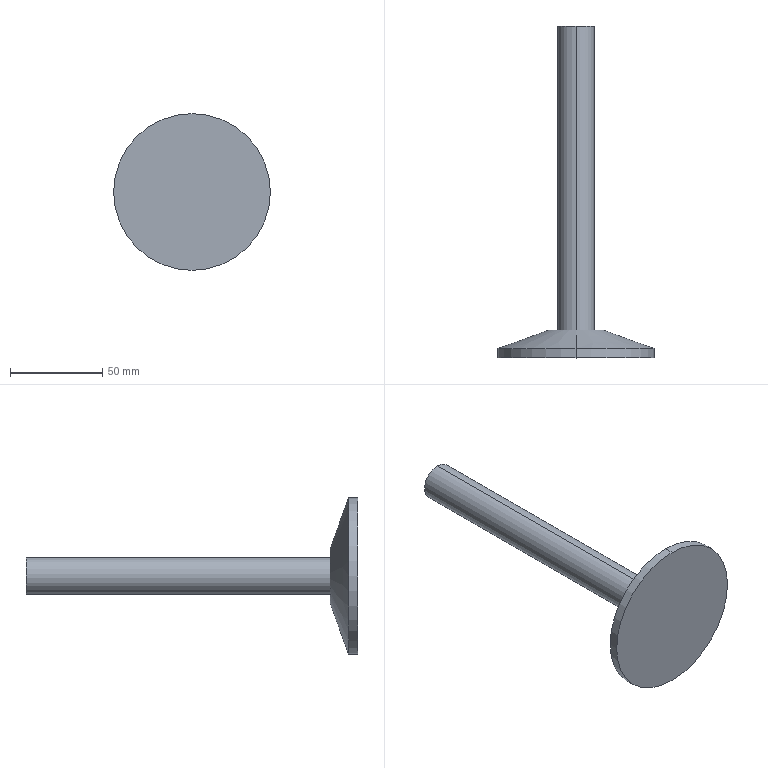Part | SolidWorks | features BaseBody 1 | 1 solid | 9 faces | box 85 x 180 x 85 mm | volume 108156 mm3 | cylinder 4 | plane 3 | cone 2 | commonest cylinder face diameters 20 x2 85 x2
STEP:
#1=CARTESIAN_POINT('',(0.,0.,42.5));
#2=VERTEX_POINT('',#1);
#3=CARTESIAN_POINT('',(0.,0.,-42.5));
#4=VERTEX_POINT('',#3);
#5=CARTESIAN_POINT('',(0.,0.,0.));
#6=DIRECTION('',(0.,1.,0.));
#7=DIRECTION('',(0.,0.,1.));
#8=AXIS2_PLACEMENT_3D('',#5,#6,#7);
#9=CIRCLE('',#8,42.5);
#10=EDGE_CURVE('',#2,#4,#9,.T.);
#11=ORIENTED_EDGE('',*,*,#10,.T.);
#12=CARTESIAN_POINT('',(0.,5.,-42.5));
#13=VERTEX_POINT('',#12);
#14=CARTESIAN_POINT('',(0.,86.546,-42.5));
#15=DIRECTION('',(0.,1.,0.));
#16=VECTOR('',#15,1000.);
#17=LINE('',#14,#16);
#18=EDGE_CURVE('',#4,#13,#17,.T.);
#19=ORIENTED_EDGE('',*,*,#18,.T.);
#20=CARTESIAN_POINT('',(0.,5.,42.5));
#21=VERTEX_POINT('',#20);
#22=CARTESIAN_POINT('',(0.,5.,0.));
#23=DIRECTION('',(0.,-1.,0.));
#24=DIRECTION('',(0.,0.,1.));
#25=AXIS2_PLACEMENT_3D('',#22,#23,#24);
#26=CIRCLE('',#25,42.5);
#27=EDGE_CURVE('',#13,#21,#26,.T.);
#28=ORIENTED_EDGE('',*,*,#27,.T.);
#29=CARTESIAN_POINT('',(0.,86.546,42.5));
#30=DIRECTION('',(0.,1.,0.));
#31=VECTOR('',#30,1000.);
#32=LINE('',#29,#31);
#33=EDGE_CURVE('',#2,#21,#32,.T.);
#34=ORIENTED_EDGE('',*,*,#33,.F.);
#35=EDGE_LOOP('',(#11,#19,#28,#34));
#36=FACE_OUTER_BOUND('',#35,.T.);
#37=CARTESIAN_POINT('',(0.,86.546,0.));
#38=DIRECTION('',(0.,1.,0.));
#39=DIRECTION('',(0.,0.,1.));
#40=AXIS2_PLACEMENT_3D('',#37,#38,#39);
#41=CYLINDRICAL_SURFACE('',#40,42.5);
#42=ADVANCED_FACE('',(#36),#41,.T.);
#43=CARTESIAN_POINT('',(0.,15.,-15.));
#44=VERTEX_POINT('',#43);
#45=CARTESIAN_POINT('',(0.,15.,15.));
#46=VERTEX_POINT('',#45);
#47=CARTESIAN_POINT('',(0.,15.,0.));
#48=DIRECTION('',(0.,-1.,0.));
#49=DIRECTION('',(0.,0.,-1.));
#50=AXIS2_PLACEMENT_3D('',#47,#48,#49);
#51=CIRCLE('',#50,15.);
#52=EDGE_CURVE('',#44,#46,#51,.T.);
#53=ORIENTED_EDGE('',*,*,#52,.T.);
#54=CARTESIAN_POINT('',(0.,5.,42.5));
#55=DIRECTION('',(0.,-0.3417,0.9398));
#56=VECTOR('',#55,1000.);
#57=LINE('',#54,#56);
#58=EDGE_CURVE('',#46,#21,#57,.T.);
#59=ORIENTED_EDGE('',*,*,#58,.T.);
#60=ORIENTED_EDGE('',*,*,#27,.F.);
#61=CARTESIAN_POINT('',(0.,5.,-42.5));
#62=DIRECTION('',(0.,-0.3417,-0.9398));
#63=VECTOR('',#62,1000.);
#64=LINE('',#61,#63);
#65=EDGE_CURVE('',#44,#13,#64,.T.);
#66=ORIENTED_EDGE('',*,*,#65,.F.);
#67=EDGE_LOOP('',(#53,#59,#60,#66));
#68=FACE_OUTER_BOUND('',#67,.T.);
#69=CARTESIAN_POINT('',(0.,5.,0.));
#70=DIRECTION('',(0.,-1.,0.));
#71=DIRECTION('',(0.,0.,-1.));
#72=AXIS2_PLACEMENT_3D('',#69,#70,#71);
#73=CONICAL_SURFACE('',#72,42.5,1.222);
#74=ADVANCED_FACE('',(#68),#73,.T.);
#75=CARTESIAN_POINT('',(0.,15.,10.));
#76=VERTEX_POINT('',#75);
#77=CARTESIAN_POINT('',(0.,15.,-10.));
#78=VERTEX_POINT('',#77);
#79=CARTESIAN_POINT('',(0.,15.,0.));
#80=DIRECTION('',(0.,1.,0.));
#81=DIRECTION('',(0.,0.,1.));
#82=AXIS2_PLACEMENT_3D('',#79,#80,#81);
#83=CIRCLE('',#82,10.);
#84=EDGE_CURVE('',#76,#78,#83,.T.);
#85=ORIENTED_EDGE('',*,*,#84,.T.);
#86=CARTESIAN_POINT('',(0.,180.,-10.));
#87=VERTEX_POINT('',#86);
#88=CARTESIAN_POINT('',(0.,86.546,-10.));
#89=DIRECTION('',(0.,1.,0.));
#90=VECTOR('',#89,1000.);
#91=LINE('',#88,#90);
#92=EDGE_CURVE('',#78,#87,#91,.T.);
#93=ORIENTED_EDGE('',*,*,#92,.T.);
#94=CARTESIAN_POINT('',(0.,180.,10.));
#95=VERTEX_POINT('',#94);
#96=CARTESIAN_POINT('',(0.,180.,0.));
#97=DIRECTION('',(0.,-1.,0.));
#98=DIRECTION('',(0.,0.,1.));
#99=AXIS2_PLACEMENT_3D('',#96,#97,#98);
#100=CIRCLE('',#99,10.);
#101=EDGE_CURVE('',#87,#95,#100,.T.);
#102=ORIENTED_EDGE('',*,*,#101,.T.);
#103=CARTESIAN_POINT('',(0.,86.546,10.));
#104=DIRECTION('',(0.,1.,0.));
#105=VECTOR('',#104,1000.);
#106=LINE('',#103,#105);
#107=EDGE_CURVE('',#76,#95,#106,.T.);
#108=ORIENTED_EDGE('',*,*,#107,.F.);
#109=EDGE_LOOP('',(#85,#93,#102,#108));
#110=FACE_OUTER_BOUND('',#109,.T.);
#111=CARTESIAN_POINT('',(0.,86.546,0.));
#112=DIRECTION('',(0.,1.,0.));
#113=DIRECTION('',(0.,0.,1.));
#114=AXIS2_PLACEMENT_3D('',#111,#112,#113);
#115=CYLINDRICAL_SURFACE('',#114,10.);
#116=ADVANCED_FACE('',(#110),#115,.T.);
#117=ORIENTED_EDGE('',*,*,#10,.F.);
#118=CARTESIAN_POINT('',(0.,0.,0.));
#119=DIRECTION('',(0.,1.,0.));
#120=DIRECTION('',(0.,0.,1.));
#121=AXIS2_PLACEMENT_3D('',#118,#119,#120);
#122=CIRCLE('',#121,42.5);
#123=EDGE_CURVE('',#4,#2,#122,.T.);
#124=ORIENTED_EDGE('',*,*,#123,.F.);
#125=EDGE_LOOP('',(#117,#124));
#126=FACE_OUTER_BOUND('',#125,.T.);
#127=CARTESIAN_POINT('',(0.,0.,0.));
#128=DIRECTION('',(0.,1.,0.));
#129=DIRECTION('',(0.,0.,1.));
#130=AXIS2_PLACEMENT_3D('',#127,#128,#129);
#131=PLANE('',#130);
#132=ADVANCED_FACE('',(#126),#131,.F.);
#133=ORIENTED_EDGE('',*,*,#18,.F.);
#134=ORIENTED_EDGE('',*,*,#123,.T.);
#135=ORIENTED_EDGE('',*,*,#33,.T.);
#136=CARTESIAN_POINT('',(0.,5.,0.));
#137=DIRECTION('',(0.,-1.,0.));
#138=DIRECTION('',(0.,0.,1.));
#139=AXIS2_PLACEMENT_3D('',#136,#137,#138);
#140=CIRCLE('',#139,42.5);
#141=EDGE_CURVE('',#21,#13,#140,.T.);
#142=ORIENTED_EDGE('',*,*,#141,.T.);
#143=EDGE_LOOP('',(#133,#134,#135,#142));
#144=FACE_OUTER_BOUND('',#143,.T.);
#145=CARTESIAN_POINT('',(0.,86.546,0.));
#146=DIRECTION('',(0.,1.,0.));
#147=DIRECTION('',(0.,0.,1.));
#148=AXIS2_PLACEMENT_3D('',#145,#146,#147);
#149=CYLINDRICAL_SURFACE('',#148,42.5);
#150=ADVANCED_FACE('',(#144),#149,.T.);
#151=ORIENTED_EDGE('',*,*,#58,.F.);
#152=CARTESIAN_POINT('',(0.,15.,0.));
#153=DIRECTION('',(0.,-1.,0.));
#154=DIRECTION('',(0.,0.,-1.));
#155=AXIS2_PLACEMENT_3D('',#152,#153,#154);
#156=CIRCLE('',#155,15.);
#157=EDGE_CURVE('',#46,#44,#156,.T.);
#158=ORIENTED_EDGE('',*,*,#157,.T.);
#159=ORIENTED_EDGE('',*,*,#65,.T.);
#160=ORIENTED_EDGE('',*,*,#141,.F.);
#161=EDGE_LOOP('',(#151,#158,#159,#160));
#162=FACE_OUTER_BOUND('',#161,.T.);
#163=CARTESIAN_POINT('',(0.,5.,0.));
#164=DIRECTION('',(0.,-1.,0.));
#165=DIRECTION('',(0.,0.,-1.));
#166=AXIS2_PLACEMENT_3D('',#163,#164,#165);
#167=CONICAL_SURFACE('',#166,42.5,1.222);
#168=ADVANCED_FACE('',(#162),#167,.T.);
#169=ORIENTED_EDGE('',*,*,#52,.F.);
#170=ORIENTED_EDGE('',*,*,#157,.F.);
#171=EDGE_LOOP('',(#169,#170));
#172=FACE_OUTER_BOUND('',#171,.T.);
#173=ORIENTED_EDGE('',*,*,#84,.F.);
#174=CARTESIAN_POINT('',(0.,15.,0.));
#175=DIRECTION('',(0.,1.,0.));
#176=DIRECTION('',(0.,0.,1.));
#177=AXIS2_PLACEMENT_3D('',#174,#175,#176);
#178=CIRCLE('',#177,10.);
#179=EDGE_CURVE('',#78,#76,#178,.T.);
#180=ORIENTED_EDGE('',*,*,#179,.F.);
#181=EDGE_LOOP('',(#173,#180));
#182=FACE_BOUND('',#181,.T.);
#183=CARTESIAN_POINT('',(15.,15.,0.));
#184=DIRECTION('',(0.,-1.,0.));
#185=DIRECTION('',(0.,0.,-1.));
#186=AXIS2_PLACEMENT_3D('',#183,#184,#185);
#187=PLANE('',#186);
#188=ADVANCED_FACE('',(#172,#182),#187,.F.);
#189=ORIENTED_EDGE('',*,*,#92,.F.);
#190=ORIENTED_EDGE('',*,*,#179,.T.);
#191=ORIENTED_EDGE('',*,*,#107,.T.);
#192=CARTESIAN_POINT('',(0.,180.,0.));
#193=DIRECTION('',(0.,-1.,0.));
#194=DIRECTION('',(0.,0.,1.));
#195=AXIS2_PLACEMENT_3D('',#192,#193,#194);
#196=CIRCLE('',#195,10.);
#197=EDGE_CURVE('',#95,#87,#196,.T.);
#198=ORIENTED_EDGE('',*,*,#197,.T.);
#199=EDGE_LOOP('',(#189,#190,#191,#198));
#200=FACE_OUTER_BOUND('',#199,.T.);
#201=CARTESIAN_POINT('',(0.,86.546,0.));
#202=DIRECTION('',(0.,1.,0.));
#203=DIRECTION('',(0.,0.,1.));
#204=AXIS2_PLACEMENT_3D('',#201,#202,#203);
#205=CYLINDRICAL_SURFACE('',#204,10.);
#206=ADVANCED_FACE('',(#200),#205,.T.);
#207=ORIENTED_EDGE('',*,*,#197,.F.);
#208=ORIENTED_EDGE('',*,*,#101,.F.);
#209=EDGE_LOOP('',(#207,#208));
#210=FACE_OUTER_BOUND('',#209,.T.);
#211=CARTESIAN_POINT('',(10.,180.,0.));
#212=DIRECTION('',(0.,-1.,0.));
#213=DIRECTION('',(0.,0.,-1.));
#214=AXIS2_PLACEMENT_3D('',#211,#212,#213);
#215=PLANE('',#214);
#216=ADVANCED_FACE('',(#210),#215,.F.);
#217=CLOSED_SHELL('',(#42,#74,#116,#132,#150,#168,#188,#206,#216));
#218=MANIFOLD_SOLID_BREP('',#217);
#219=CARTESIAN_POINT('',(0.,0.,0.));
#220=DIRECTION('',(0.,0.,1.));
#221=DIRECTION('',(1.,0.,0.));
#222=AXIS2_PLACEMENT_3D('',#219,#220,#221);
#223=(LENGTH_UNIT()NAMED_UNIT(*)SI_UNIT(.MILLI.,.METRE.));
#224=UNCERTAINTY_MEASURE_WITH_UNIT(LENGTH_MEASURE(0.00001),#223,'','');
#225=(NAMED_UNIT(*)PLANE_ANGLE_UNIT()SI_UNIT($,.RADIAN.));
#226=(NAMED_UNIT(*)SI_UNIT($,.STERADIAN.)SOLID_ANGLE_UNIT());
#227=(GEOMETRIC_REPRESENTATION_CONTEXT(3)GLOBAL_UNCERTAINTY_ASSIGNED_CONTEXT((#224))GLOBAL_UNIT_ASSIGNED_CONTEXT((#223,#225,#226))REPRESENTATION_CONTEXT('',''));
#228=ADVANCED_BREP_SHAPE_REPRESENTATION('',(#218,#222),#227);